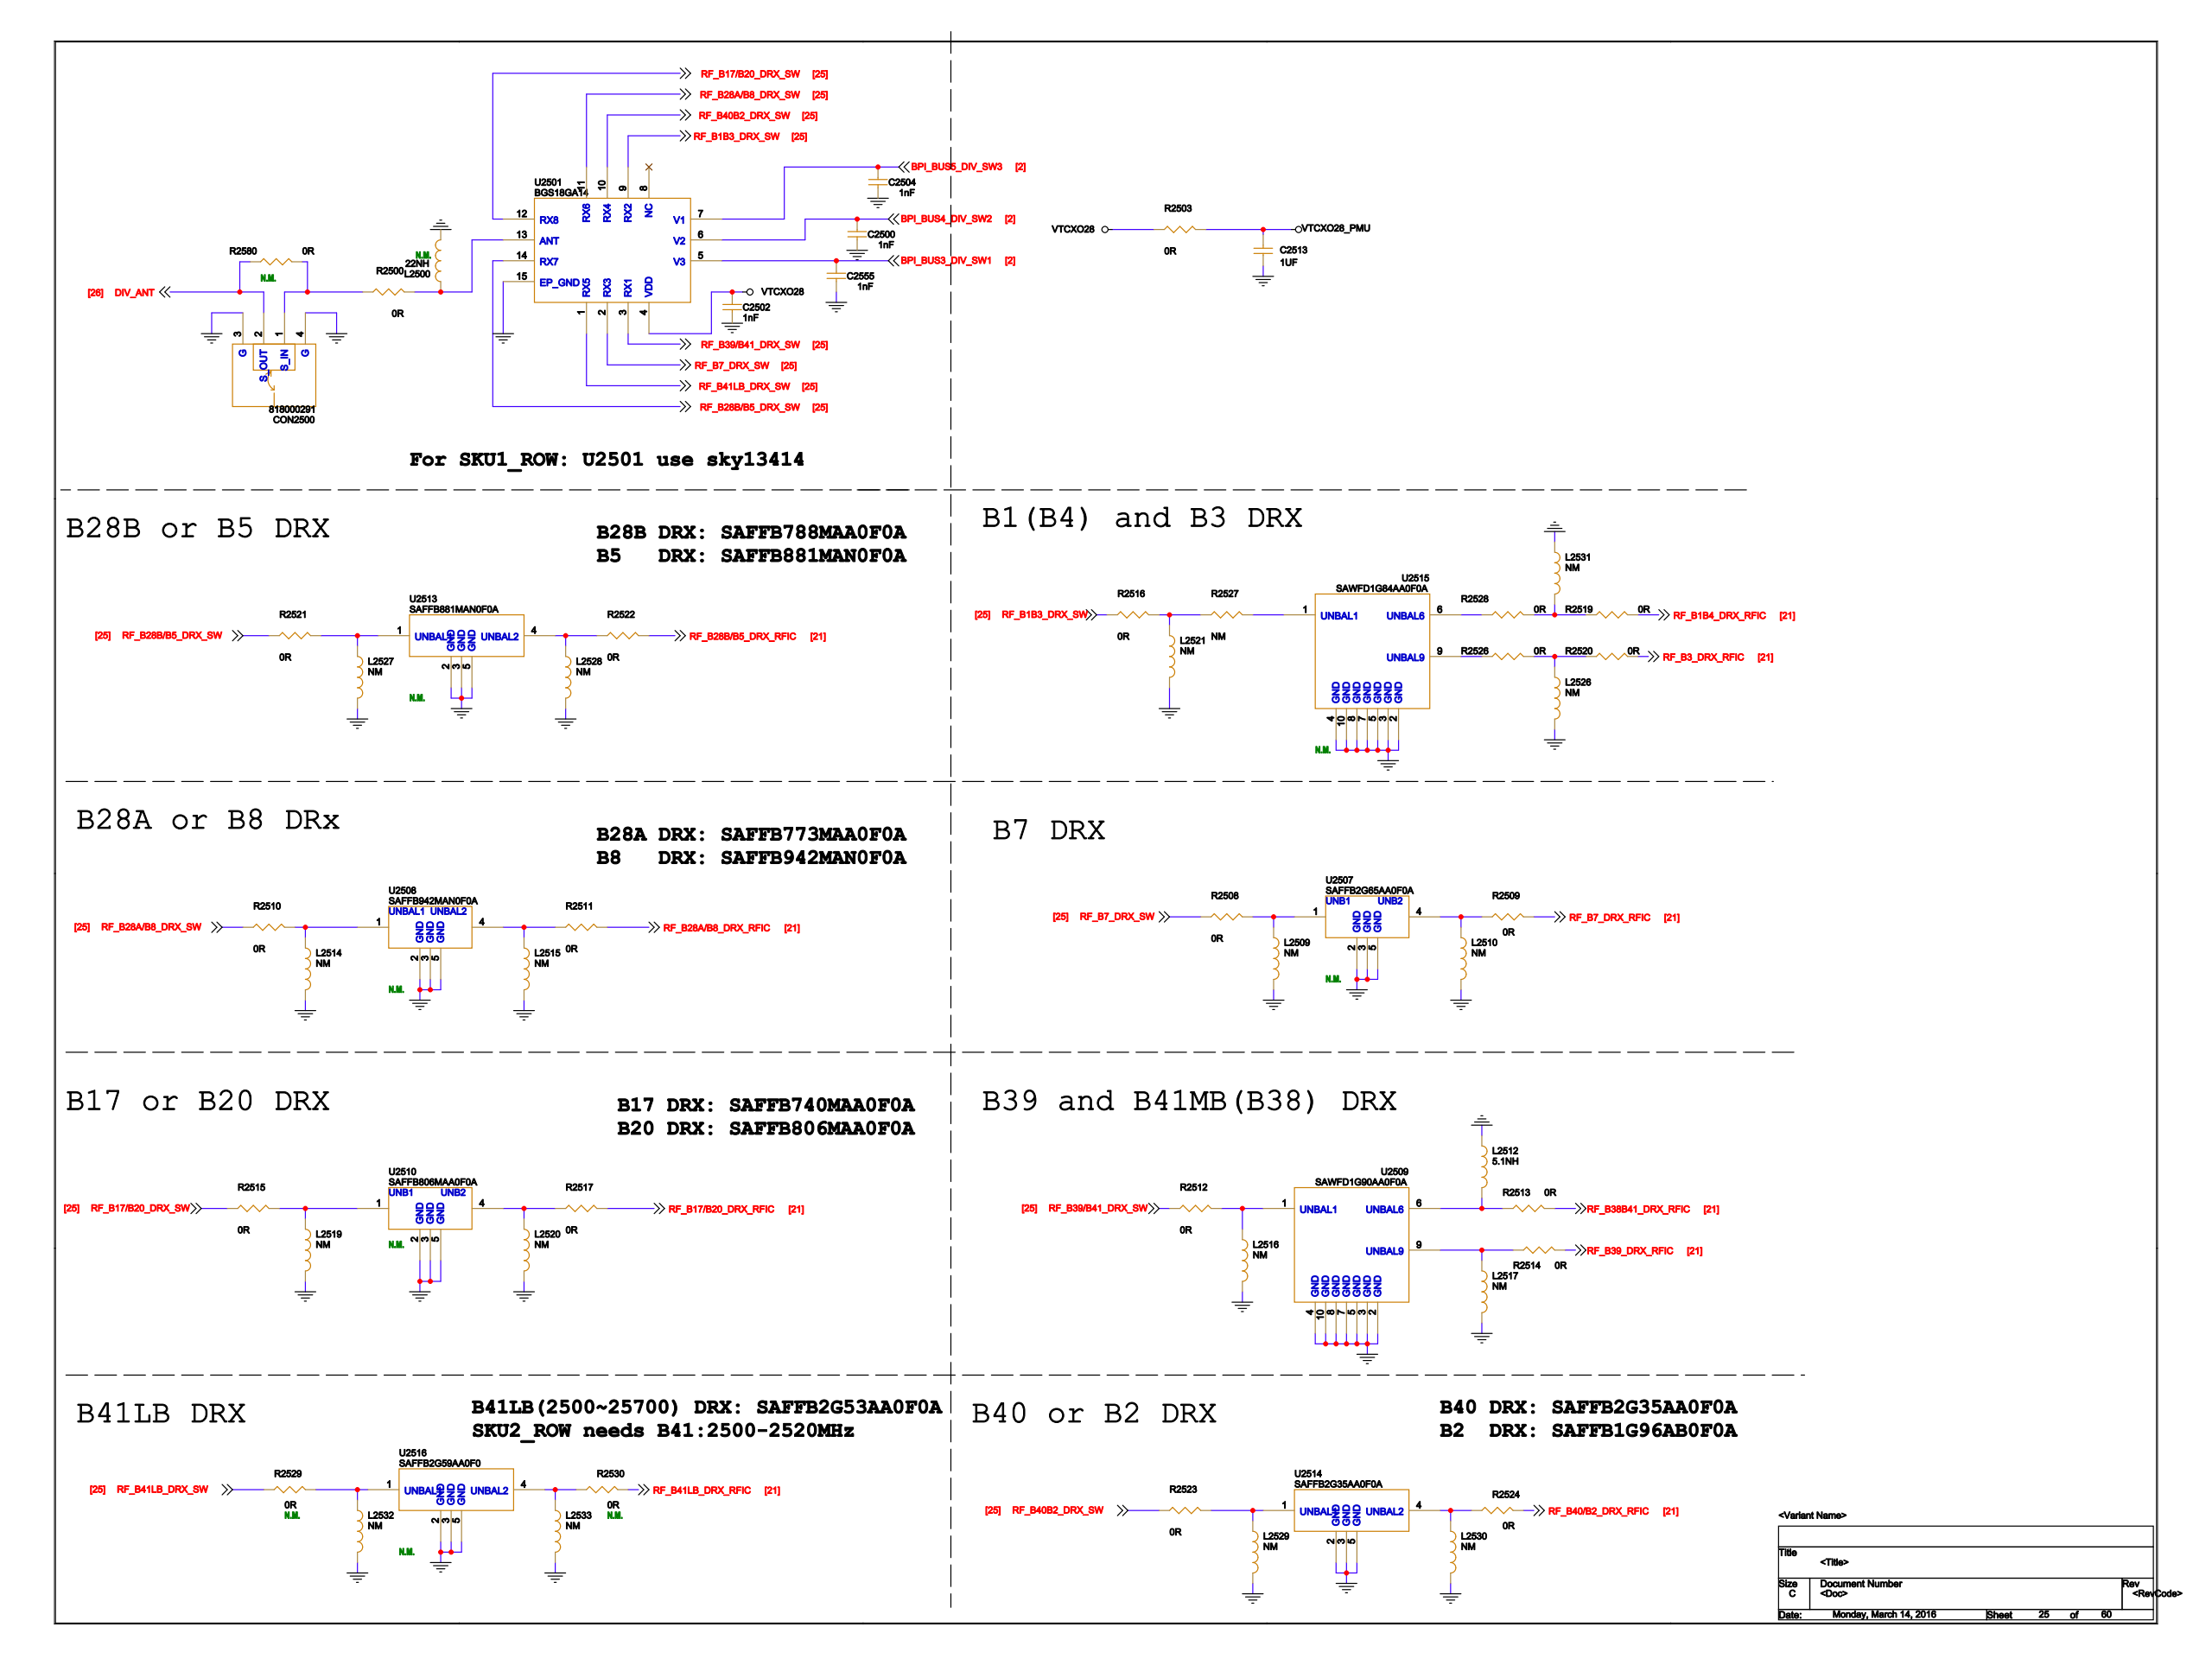Circuit board | Cadence Allegro | 1088 parts | 793 nets | one sheet of the schematic
Parts on this sheet (reference | value | footprint):
C2500 | 1nF | C0201
C2502 | 1nF | C0201
C2504 | 1nF | C0201
C2513 | 1UF | C0201
C2555 | 1nF | C0201
CON2500 | 818000291 | RF_818000291
L2500
L2509 | NM | 0201_NM
L2510 | NM | 0201_NM
L2512 | 5.1nH | L0201
L2514 | NM | 0201_NM
L2515 | NM | 0201_NM
L2516 | NM | 0201_NM
L2517 | NM | 0201_NM
L2519 | NM | 0201_NM
L2520 | NM | 0201_NM
L2521 | NM | 0201_NM
L2526 | NM | 0201_NM
L2527 | NM | 0201_NM
L2528 | NM | 0201_NM
L2529 | NM | 0201_NM
L2530 | NM | 0201_NM
L2531 | NM | 0201_NM
L2532 | NM | 0201_NM
L2533 | NM | 0201_NM
R2500 | 0R | R0201
R2503 | 0R | R0201
R2508 | 0R | R0201
R2509 | 0R | R0201
R2510 | 0R | R0201
R2511 | 0R | R0201
R2512 | 0R | R0201
R2513 | 0R | R0201
R2514 | 0R | R0201
R2515 | 0R | R0201
R2516 | 0R | R0201
R2517 | 0R | R0201
R2519 | 0R | R0201
R2520 | 0R | R0201
R2521 | 0R | R0201
R2522 | 0R | R0201
R2523 | 0R | R0201
R2524 | 0R | R0201
R2526 | 0R | R0201
R2527 | NM | 0201_NM
R2528 | 0R | R0201
R2529
R2530
R2580
U2501 | BGS18GA14 | TSLP14_2X2X0P75
U2507
U2508
U2509 | SAWFD1G90AA0F0A | SAW1511_H0P6_MURATA
U2510
U2513
U2514 | SAFFB2G35AA0F0A | SAW1109_H0P6_MURATA
U2515
U2516
Nets of these parts (net: part-pin ...):
GND: C2500-2 C2502-2 C2504-2 C2513-1 C2555-2 CON2500-3 CON2500-4 L2500-2 L2509-2 L2510-2 L2512-1 L2514-2 L2515-2 L2516-2 L2517-2 L2519-2 L2520-2 L2521-2 L2526-2 L2527-2 L2528-2 L2529-2 L2530-2 L2531-1 L2532-2 L2533-2 U2501-15 U2507-2 U2507-3 U2507-5 U2508-2 U2508-3 U2508-5 U2509-2 U2509-3 U2509-4 U2509-5 U2509-7 U2509-8 U2509-10 U2510-2 U2510-3 U2510-5 U2513-2 U2513-3 U2513-5 U2514-2 U2514-3 U2514-5 U2515-2 U2515-3 U2515-4 U2515-5 U2515-7 U2515-8 U2515-10 U2516-2 U2516-3 U2516-5
N57623: L2512-2 R2513-1 U2509-6
N57721: CON2500-1 R2500-2 R2580-2
DIV_ANT: CON2500-2 R2580-1
N57437: L2500-1 R2500-1 U2501-13
RF_B39/B41_DRX_SW: R2512-1 U2501-3
RF_B1B3_DRX_SW: R2516-1 U2501-9
RF_B7_DRX_SW: R2508-1 U2501-2
RF_B40B2_DRX_SW: R2523-1 U2501-10
RF_B41LB_DRX_SW: R2529-1 U2501-1
RF_B28A/B8_DRX_SW: R2510-1 U2501-11
RF_B28B/B5_DRX_SW: R2521-1 U2501-14
RF_B17/B20_DRX_SW: R2515-1 U2501-12
BPI_BUS5_DIV_SW3: C2504-1 U2501-7
BPI_BUS4_DIV_SW2: C2500-1 U2501-6
BPI_BUS3_DIV_SW1: C2555-1 U2501-5
VTCXO28: C2502-1 R2503-1 U2501-4
VTCXO28_PMU: C2513-2 R2503-2
N57579: L2509-1 R2508-2 U2507-1
N57587: L2510-1 R2509-1 U2507-4
N57495: L2514-1 R2510-2 U2508-1
N57505: L2515-1 R2511-1 U2508-4
N32758654: L2516-1 R2512-2 U2509-1
N57629: L2517-1 R2514-1 U2509-9
N57515: L2519-1 R2515-2 U2510-1
N57523: L2520-1 R2517-1 U2510-4
N33280928: L2521-1 R2516-2 R2527-1
N33280910: L2526-1 R2520-1 R2526-1
N33377225: L2527-1 R2521-2 U2513-1
N33377217: L2528-1 R2522-1 U2513-4
N57663: L2529-1 R2523-2 U2514-1
N33521535: L2530-1 R2524-1 U2514-4
N33281069: L2531-2 R2519-2 R2528-1
N33532368: L2532-1 R2529-2 U2516-1
N33531869: L2533-1 R2530-1 U2516-4
N33281009: R2527-2 U2515-1
RF_B17/B20_DRX_RFIC: R2517-2
RF_B38B41_DRX_RFIC: R2513-2
RF_B41LB_DRX_RFIC: R2530-2
RF_B3_DRX_RFIC: R2520-2
RF_B28B/B5_DRX_RFIC: R2522-2
RF_B39_DRX_RFIC: R2514-2
RF_B1B4_DRX_RFIC: R2519-1
RF_B28A/B8_DRX_RFIC: R2511-2
RF_B7_DRX_RFIC: R2509-2
RF_B40/B2_DRX_RFIC: R2524-2
N33281049: R2528-2 U2515-6
N33280996: R2526-2 U2515-9